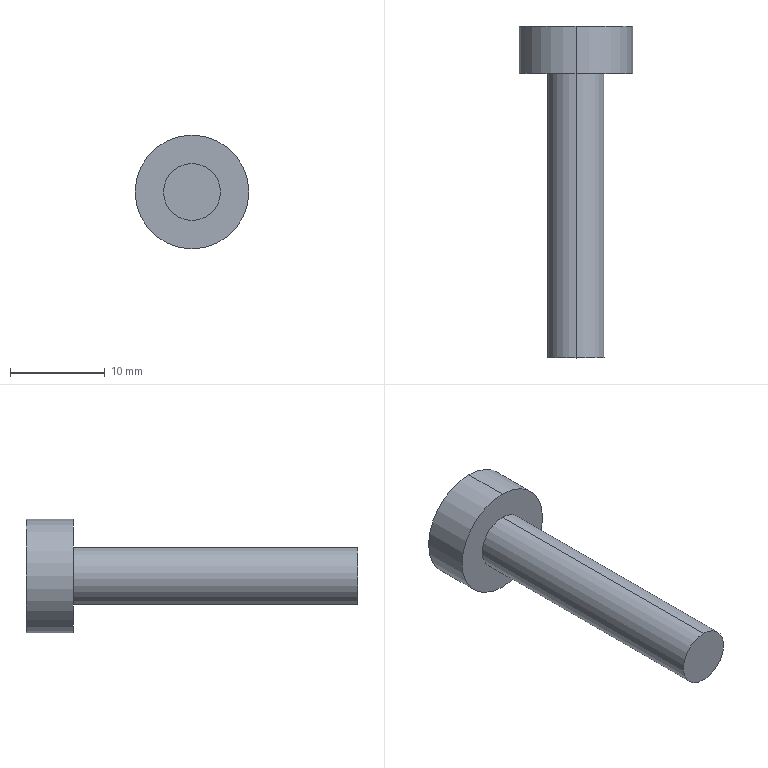Part | STEP file | 1 solid | 7 faces | box 12 x 35 x 12 mm | volume 1414 mm3 | cylinder 4 | plane 3 | commonest cylinder face diameters 6 x2 12 x2
STEP:
#1=CARTESIAN_POINT('',(0.,0.,0.));
#2=DIRECTION('',(0.,0.,1.));
#3=DIRECTION('',(1.,0.,0.));
#4=AXIS2_PLACEMENT_3D('',#1,#2,#3);
#5=CARTESIAN_POINT('',(0.,35.,-6.));
#6=VERTEX_POINT('',#5);
#7=CARTESIAN_POINT('',(0.,35.,6.));
#8=VERTEX_POINT('',#7);
#9=CARTESIAN_POINT('',(0.,35.,0.));
#10=DIRECTION('',(0.,-1.,0.));
#11=DIRECTION('',(0.,0.,-1.));
#12=AXIS2_PLACEMENT_3D('',#9,#10,#11);
#13=CIRCLE('',#12,6.);
#14=CARTESIAN_POINT('',(0.,0.,0.));
#15=DIRECTION('',(0.,-1.,0.));
#16=DIRECTION('',(0.,0.,-1.));
#17=AXIS2_PLACEMENT_3D('',#14,#15,#16);
#18=CYLINDRICAL_SURFACE('',#17,6.);
#19=CARTESIAN_POINT('',(0.,-35.));
#20=DIRECTION('',(1.,0.));
#21=VECTOR('',#20,1.);
#22=LINE('',#19,#21);
#23=(GEOMETRIC_REPRESENTATION_CONTEXT(2)PARAMETRIC_REPRESENTATION_CONTEXT()REPRESENTATION_CONTEXT('',''));
#24=DEFINITIONAL_REPRESENTATION('',(#22),#23);
#25=PCURVE('',#18,#24);
#26=CARTESIAN_POINT('',(6.,35.,0.));
#27=DIRECTION('',(0.,1.,0.));
#28=DIRECTION('',(0.,0.,1.));
#29=AXIS2_PLACEMENT_3D('',#26,#27,#28);
#30=PLANE('',#29);
#31=CARTESIAN_POINT('',(-6.,-6.));
#32=CARTESIAN_POINT('',(-6.,4.392));
#33=CARTESIAN_POINT('',(3.,-0.8038));
#34=CARTESIAN_POINT('',(12.,-6.));
#35=CARTESIAN_POINT('',(3.,-11.196));
#36=CARTESIAN_POINT('',(-6.,-16.392));
#37=CARTESIAN_POINT('',(-6.,-6.));
#38=(BOUNDED_CURVE()B_SPLINE_CURVE(2,(#31,#32,#33,#34,#35,#36,#37),.UNSPECIFIED.,.T.,.F.)B_SPLINE_CURVE_WITH_KNOTS((1,2,2,2,2,1),(-2.094,0.,2.094,4.189,6.283,8.378),.UNSPECIFIED.)CURVE()GEOMETRIC_REPRESENTATION_ITEM()RATIONAL_B_SPLINE_CURVE((1.,0.5,1.,0.5,1.,0.5,1.))REPRESENTATION_ITEM(''));
#39=(GEOMETRIC_REPRESENTATION_CONTEXT(2)PARAMETRIC_REPRESENTATION_CONTEXT()REPRESENTATION_CONTEXT('',''));
#40=DEFINITIONAL_REPRESENTATION('',(#38),#39);
#41=PCURVE('',#30,#40);
#42=SURFACE_CURVE('',#13,(#25,#41),.PCURVE_S1.);
#43=EDGE_CURVE('',#6,#8,#42,.T.);
#44=ORIENTED_EDGE('',*,*,#43,.T.);
#45=CARTESIAN_POINT('',(0.,30.,6.));
#46=VERTEX_POINT('',#45);
#47=CARTESIAN_POINT('',(0.,0.,6.));
#48=DIRECTION('',(0.,-1.,0.));
#49=VECTOR('',#48,1.);
#50=LINE('',#47,#49);
#51=CARTESIAN_POINT('',(3.142,0.));
#52=DIRECTION('',(0.,1.));
#53=VECTOR('',#52,1.);
#54=LINE('',#51,#53);
#55=(GEOMETRIC_REPRESENTATION_CONTEXT(2)PARAMETRIC_REPRESENTATION_CONTEXT()REPRESENTATION_CONTEXT('',''));
#56=DEFINITIONAL_REPRESENTATION('',(#54),#55);
#57=PCURVE('',#18,#56);
#58=CARTESIAN_POINT('',(0.,0.,0.));
#59=DIRECTION('',(0.,-1.,0.));
#60=DIRECTION('',(0.,0.,-1.));
#61=AXIS2_PLACEMENT_3D('',#58,#59,#60);
#62=CYLINDRICAL_SURFACE('',#61,6.);
#63=CARTESIAN_POINT('',(3.142,0.));
#64=DIRECTION('',(0.,1.));
#65=VECTOR('',#64,1.);
#66=LINE('',#63,#65);
#67=(GEOMETRIC_REPRESENTATION_CONTEXT(2)PARAMETRIC_REPRESENTATION_CONTEXT()REPRESENTATION_CONTEXT('',''));
#68=DEFINITIONAL_REPRESENTATION('',(#66),#67);
#69=PCURVE('',#62,#68);
#70=SURFACE_CURVE('',#50,(#57,#69),.PCURVE_S1.);
#71=EDGE_CURVE('',#8,#46,#70,.T.);
#72=ORIENTED_EDGE('',*,*,#71,.T.);
#73=CARTESIAN_POINT('',(0.,30.,-6.));
#74=VERTEX_POINT('',#73);
#75=CARTESIAN_POINT('',(0.,30.,0.));
#76=DIRECTION('',(0.,-1.,0.));
#77=DIRECTION('',(0.,0.,-1.));
#78=AXIS2_PLACEMENT_3D('',#75,#76,#77);
#79=CIRCLE('',#78,6.);
#80=CARTESIAN_POINT('',(0.,-30.));
#81=DIRECTION('',(1.,0.));
#82=VECTOR('',#81,1.);
#83=LINE('',#80,#82);
#84=(GEOMETRIC_REPRESENTATION_CONTEXT(2)PARAMETRIC_REPRESENTATION_CONTEXT()REPRESENTATION_CONTEXT('',''));
#85=DEFINITIONAL_REPRESENTATION('',(#83),#84);
#86=PCURVE('',#18,#85);
#87=CARTESIAN_POINT('',(3.,30.,0.));
#88=DIRECTION('',(0.,-1.,0.));
#89=DIRECTION('',(0.,0.,-1.));
#90=AXIS2_PLACEMENT_3D('',#87,#88,#89);
#91=PLANE('',#90);
#92=CARTESIAN_POINT('',(0.,-3.));
#93=DIRECTION('',(1.,0.));
#94=AXIS2_PLACEMENT_2D('',#92,#93);
#95=CIRCLE('',#94,6.);
#96=(GEOMETRIC_REPRESENTATION_CONTEXT(2)PARAMETRIC_REPRESENTATION_CONTEXT()REPRESENTATION_CONTEXT('',''));
#97=DEFINITIONAL_REPRESENTATION('',(#95),#96);
#98=PCURVE('',#91,#97);
#99=SURFACE_CURVE('',#79,(#86,#98),.PCURVE_S1.);
#100=EDGE_CURVE('',#74,#46,#99,.T.);
#101=ORIENTED_EDGE('',*,*,#100,.F.);
#102=CARTESIAN_POINT('',(0.,0.,-6.));
#103=DIRECTION('',(0.,-1.,0.));
#104=VECTOR('',#103,1.);
#105=LINE('',#102,#104);
#106=CARTESIAN_POINT('',(0.,0.));
#107=DIRECTION('',(0.,1.));
#108=VECTOR('',#107,1.);
#109=LINE('',#106,#108);
#110=(GEOMETRIC_REPRESENTATION_CONTEXT(2)PARAMETRIC_REPRESENTATION_CONTEXT()REPRESENTATION_CONTEXT('',''));
#111=DEFINITIONAL_REPRESENTATION('',(#109),#110);
#112=PCURVE('',#18,#111);
#113=CARTESIAN_POINT('',(6.283,0.));
#114=DIRECTION('',(0.,1.));
#115=VECTOR('',#114,1.);
#116=LINE('',#113,#115);
#117=(GEOMETRIC_REPRESENTATION_CONTEXT(2)PARAMETRIC_REPRESENTATION_CONTEXT()REPRESENTATION_CONTEXT('',''));
#118=DEFINITIONAL_REPRESENTATION('',(#116),#117);
#119=PCURVE('',#62,#118);
#120=SURFACE_CURVE('',#105,(#112,#119),.PCURVE_S1.);
#121=EDGE_CURVE('',#6,#74,#120,.T.);
#122=ORIENTED_EDGE('',*,*,#121,.F.);
#123=EDGE_LOOP('',(#44,#72,#101,#122));
#124=FACE_BOUND('',#123,.T.);
#125=ADVANCED_FACE('',(#124),#18,.T.);
#126=CARTESIAN_POINT('',(0.,30.,-3.));
#127=VERTEX_POINT('',#126);
#128=CARTESIAN_POINT('',(0.,30.,3.));
#129=VERTEX_POINT('',#128);
#130=CARTESIAN_POINT('',(0.,30.,0.));
#131=DIRECTION('',(0.,-1.,0.));
#132=DIRECTION('',(0.,0.,-1.));
#133=AXIS2_PLACEMENT_3D('',#130,#131,#132);
#134=CIRCLE('',#133,3.);
#135=CARTESIAN_POINT('',(0.,0.,0.));
#136=DIRECTION('',(0.,-1.,0.));
#137=DIRECTION('',(0.,0.,-1.));
#138=AXIS2_PLACEMENT_3D('',#135,#136,#137);
#139=CYLINDRICAL_SURFACE('',#138,3.);
#140=CARTESIAN_POINT('',(0.,-30.));
#141=DIRECTION('',(1.,0.));
#142=VECTOR('',#141,1.);
#143=LINE('',#140,#142);
#144=(GEOMETRIC_REPRESENTATION_CONTEXT(2)PARAMETRIC_REPRESENTATION_CONTEXT()REPRESENTATION_CONTEXT('',''));
#145=DEFINITIONAL_REPRESENTATION('',(#143),#144);
#146=PCURVE('',#139,#145);
#147=CARTESIAN_POINT('',(0.,-3.));
#148=DIRECTION('',(1.,0.));
#149=AXIS2_PLACEMENT_2D('',#147,#148);
#150=CIRCLE('',#149,3.);
#151=(GEOMETRIC_REPRESENTATION_CONTEXT(2)PARAMETRIC_REPRESENTATION_CONTEXT()REPRESENTATION_CONTEXT('',''));
#152=DEFINITIONAL_REPRESENTATION('',(#150),#151);
#153=PCURVE('',#91,#152);
#154=SURFACE_CURVE('',#134,(#146,#153),.PCURVE_S1.);
#155=EDGE_CURVE('',#127,#129,#154,.T.);
#156=ORIENTED_EDGE('',*,*,#155,.T.);
#157=CARTESIAN_POINT('',(0.,0.,3.));
#158=VERTEX_POINT('',#157);
#159=CARTESIAN_POINT('',(0.,0.,3.));
#160=DIRECTION('',(0.,-1.,0.));
#161=VECTOR('',#160,1.);
#162=LINE('',#159,#161);
#163=CARTESIAN_POINT('',(3.142,0.));
#164=DIRECTION('',(0.,1.));
#165=VECTOR('',#164,1.);
#166=LINE('',#163,#165);
#167=(GEOMETRIC_REPRESENTATION_CONTEXT(2)PARAMETRIC_REPRESENTATION_CONTEXT()REPRESENTATION_CONTEXT('',''));
#168=DEFINITIONAL_REPRESENTATION('',(#166),#167);
#169=PCURVE('',#139,#168);
#170=CARTESIAN_POINT('',(0.,0.,0.));
#171=DIRECTION('',(0.,-1.,0.));
#172=DIRECTION('',(0.,0.,-1.));
#173=AXIS2_PLACEMENT_3D('',#170,#171,#172);
#174=CYLINDRICAL_SURFACE('',#173,3.);
#175=CARTESIAN_POINT('',(3.142,0.));
#176=DIRECTION('',(0.,1.));
#177=VECTOR('',#176,1.);
#178=LINE('',#175,#177);
#179=(GEOMETRIC_REPRESENTATION_CONTEXT(2)PARAMETRIC_REPRESENTATION_CONTEXT()REPRESENTATION_CONTEXT('',''));
#180=DEFINITIONAL_REPRESENTATION('',(#178),#179);
#181=PCURVE('',#174,#180);
#182=SURFACE_CURVE('',#162,(#169,#181),.PCURVE_S1.);
#183=EDGE_CURVE('',#129,#158,#182,.T.);
#184=ORIENTED_EDGE('',*,*,#183,.T.);
#185=CARTESIAN_POINT('',(0.,0.,-3.));
#186=VERTEX_POINT('',#185);
#187=CARTESIAN_POINT('',(0.,0.,0.));
#188=DIRECTION('',(0.,-1.,0.));
#189=DIRECTION('',(0.,0.,-1.));
#190=AXIS2_PLACEMENT_3D('',#187,#188,#189);
#191=CIRCLE('',#190,3.);
#192=CARTESIAN_POINT('',(0.,0.));
#193=DIRECTION('',(1.,0.));
#194=VECTOR('',#193,1.);
#195=LINE('',#192,#194);
#196=(GEOMETRIC_REPRESENTATION_CONTEXT(2)PARAMETRIC_REPRESENTATION_CONTEXT()REPRESENTATION_CONTEXT('',''));
#197=DEFINITIONAL_REPRESENTATION('',(#195),#196);
#198=PCURVE('',#139,#197);
#199=CARTESIAN_POINT('',(0.,0.,0.));
#200=DIRECTION('',(0.,-1.,0.));
#201=DIRECTION('',(0.,0.,-1.));
#202=AXIS2_PLACEMENT_3D('',#199,#200,#201);
#203=PLANE('',#202);
#204=CARTESIAN_POINT('',(0.,0.));
#205=DIRECTION('',(1.,0.));
#206=AXIS2_PLACEMENT_2D('',#204,#205);
#207=CIRCLE('',#206,3.);
#208=(GEOMETRIC_REPRESENTATION_CONTEXT(2)PARAMETRIC_REPRESENTATION_CONTEXT()REPRESENTATION_CONTEXT('',''));
#209=DEFINITIONAL_REPRESENTATION('',(#207),#208);
#210=PCURVE('',#203,#209);
#211=SURFACE_CURVE('',#191,(#198,#210),.PCURVE_S1.);
#212=EDGE_CURVE('',#186,#158,#211,.T.);
#213=ORIENTED_EDGE('',*,*,#212,.F.);
#214=CARTESIAN_POINT('',(0.,0.,-3.));
#215=DIRECTION('',(0.,-1.,0.));
#216=VECTOR('',#215,1.);
#217=LINE('',#214,#216);
#218=CARTESIAN_POINT('',(0.,0.));
#219=DIRECTION('',(0.,1.));
#220=VECTOR('',#219,1.);
#221=LINE('',#218,#220);
#222=(GEOMETRIC_REPRESENTATION_CONTEXT(2)PARAMETRIC_REPRESENTATION_CONTEXT()REPRESENTATION_CONTEXT('',''));
#223=DEFINITIONAL_REPRESENTATION('',(#221),#222);
#224=PCURVE('',#139,#223);
#225=CARTESIAN_POINT('',(6.283,0.));
#226=DIRECTION('',(0.,1.));
#227=VECTOR('',#226,1.);
#228=LINE('',#225,#227);
#229=(GEOMETRIC_REPRESENTATION_CONTEXT(2)PARAMETRIC_REPRESENTATION_CONTEXT()REPRESENTATION_CONTEXT('',''));
#230=DEFINITIONAL_REPRESENTATION('',(#228),#229);
#231=PCURVE('',#174,#230);
#232=SURFACE_CURVE('',#217,(#224,#231),.PCURVE_S1.);
#233=EDGE_CURVE('',#127,#186,#232,.T.);
#234=ORIENTED_EDGE('',*,*,#233,.F.);
#235=EDGE_LOOP('',(#156,#184,#213,#234));
#236=FACE_BOUND('',#235,.T.);
#237=ADVANCED_FACE('',(#236),#139,.T.);
#238=ORIENTED_EDGE('',*,*,#212,.T.);
#239=CARTESIAN_POINT('',(0.,0.,0.));
#240=DIRECTION('',(0.,-1.,0.));
#241=DIRECTION('',(0.,0.,-1.));
#242=AXIS2_PLACEMENT_3D('',#239,#240,#241);
#243=CIRCLE('',#242,3.);
#244=CARTESIAN_POINT('',(0.,0.));
#245=DIRECTION('',(1.,0.));
#246=AXIS2_PLACEMENT_2D('',#244,#245);
#247=CIRCLE('',#246,3.);
#248=(GEOMETRIC_REPRESENTATION_CONTEXT(2)PARAMETRIC_REPRESENTATION_CONTEXT()REPRESENTATION_CONTEXT('',''));
#249=DEFINITIONAL_REPRESENTATION('',(#247),#248);
#250=PCURVE('',#203,#249);
#251=CARTESIAN_POINT('',(0.,0.));
#252=DIRECTION('',(1.,0.));
#253=VECTOR('',#252,1.);
#254=LINE('',#251,#253);
#255=(GEOMETRIC_REPRESENTATION_CONTEXT(2)PARAMETRIC_REPRESENTATION_CONTEXT()REPRESENTATION_CONTEXT('',''));
#256=DEFINITIONAL_REPRESENTATION('',(#254),#255);
#257=PCURVE('',#174,#256);
#258=SURFACE_CURVE('',#243,(#250,#257),.PCURVE_S1.);
#259=EDGE_CURVE('',#158,#186,#258,.T.);
#260=ORIENTED_EDGE('',*,*,#259,.T.);
#261=EDGE_LOOP('',(#238,#260));
#262=FACE_BOUND('',#261,.T.);
#263=ADVANCED_FACE('',(#262),#203,.T.);
#264=ORIENTED_EDGE('',*,*,#183,.F.);
#265=CARTESIAN_POINT('',(0.,30.,0.));
#266=DIRECTION('',(0.,-1.,0.));
#267=DIRECTION('',(0.,0.,-1.));
#268=AXIS2_PLACEMENT_3D('',#265,#266,#267);
#269=CIRCLE('',#268,3.);
#270=CARTESIAN_POINT('',(0.,-30.));
#271=DIRECTION('',(1.,0.));
#272=VECTOR('',#271,1.);
#273=LINE('',#270,#272);
#274=(GEOMETRIC_REPRESENTATION_CONTEXT(2)PARAMETRIC_REPRESENTATION_CONTEXT()REPRESENTATION_CONTEXT('',''));
#275=DEFINITIONAL_REPRESENTATION('',(#273),#274);
#276=PCURVE('',#174,#275);
#277=CARTESIAN_POINT('',(0.,-3.));
#278=DIRECTION('',(1.,0.));
#279=AXIS2_PLACEMENT_2D('',#277,#278);
#280=CIRCLE('',#279,3.);
#281=(GEOMETRIC_REPRESENTATION_CONTEXT(2)PARAMETRIC_REPRESENTATION_CONTEXT()REPRESENTATION_CONTEXT('',''));
#282=DEFINITIONAL_REPRESENTATION('',(#280),#281);
#283=PCURVE('',#91,#282);
#284=SURFACE_CURVE('',#269,(#276,#283),.PCURVE_S1.);
#285=EDGE_CURVE('',#129,#127,#284,.T.);
#286=ORIENTED_EDGE('',*,*,#285,.T.);
#287=ORIENTED_EDGE('',*,*,#233,.T.);
#288=ORIENTED_EDGE('',*,*,#259,.F.);
#289=EDGE_LOOP('',(#264,#286,#287,#288));
#290=FACE_BOUND('',#289,.T.);
#291=ADVANCED_FACE('',(#290),#174,.T.);
#292=ORIENTED_EDGE('',*,*,#100,.T.);
#293=CARTESIAN_POINT('',(0.,30.,0.));
#294=DIRECTION('',(0.,-1.,0.));
#295=DIRECTION('',(0.,0.,-1.));
#296=AXIS2_PLACEMENT_3D('',#293,#294,#295);
#297=CIRCLE('',#296,6.);
#298=CARTESIAN_POINT('',(0.,-3.));
#299=DIRECTION('',(1.,0.));
#300=AXIS2_PLACEMENT_2D('',#298,#299);
#301=CIRCLE('',#300,6.);
#302=(GEOMETRIC_REPRESENTATION_CONTEXT(2)PARAMETRIC_REPRESENTATION_CONTEXT()REPRESENTATION_CONTEXT('',''));
#303=DEFINITIONAL_REPRESENTATION('',(#301),#302);
#304=PCURVE('',#91,#303);
#305=CARTESIAN_POINT('',(0.,-30.));
#306=DIRECTION('',(1.,0.));
#307=VECTOR('',#306,1.);
#308=LINE('',#305,#307);
#309=(GEOMETRIC_REPRESENTATION_CONTEXT(2)PARAMETRIC_REPRESENTATION_CONTEXT()REPRESENTATION_CONTEXT('',''));
#310=DEFINITIONAL_REPRESENTATION('',(#308),#309);
#311=PCURVE('',#62,#310);
#312=SURFACE_CURVE('',#297,(#304,#311),.PCURVE_S1.);
#313=EDGE_CURVE('',#46,#74,#312,.T.);
#314=ORIENTED_EDGE('',*,*,#313,.T.);
#315=EDGE_LOOP('',(#292,#314));
#316=FACE_BOUND('',#315,.T.);
#317=ORIENTED_EDGE('',*,*,#155,.F.);
#318=ORIENTED_EDGE('',*,*,#285,.F.);
#319=EDGE_LOOP('',(#317,#318));
#320=FACE_BOUND('',#319,.T.);
#321=ADVANCED_FACE('',(#316,#320),#91,.T.);
#322=ORIENTED_EDGE('',*,*,#71,.F.);
#323=CARTESIAN_POINT('',(0.,35.,0.));
#324=DIRECTION('',(0.,-1.,0.));
#325=DIRECTION('',(0.,0.,-1.));
#326=AXIS2_PLACEMENT_3D('',#323,#324,#325);
#327=CIRCLE('',#326,6.);
#328=CARTESIAN_POINT('',(0.,-35.));
#329=DIRECTION('',(1.,0.));
#330=VECTOR('',#329,1.);
#331=LINE('',#328,#330);
#332=(GEOMETRIC_REPRESENTATION_CONTEXT(2)PARAMETRIC_REPRESENTATION_CONTEXT()REPRESENTATION_CONTEXT('',''));
#333=DEFINITIONAL_REPRESENTATION('',(#331),#332);
#334=PCURVE('',#62,#333);
#335=CARTESIAN_POINT('',(-6.,-6.));
#336=CARTESIAN_POINT('',(-6.,4.392));
#337=CARTESIAN_POINT('',(3.,-0.8038));
#338=CARTESIAN_POINT('',(12.,-6.));
#339=CARTESIAN_POINT('',(3.,-11.196));
#340=CARTESIAN_POINT('',(-6.,-16.392));
#341=CARTESIAN_POINT('',(-6.,-6.));
#342=(BOUNDED_CURVE()B_SPLINE_CURVE(2,(#335,#336,#337,#338,#339,#340,#341),.UNSPECIFIED.,.T.,.F.)B_SPLINE_CURVE_WITH_KNOTS((1,2,2,2,2,1),(-2.094,0.,2.094,4.189,6.283,8.378),.UNSPECIFIED.)CURVE()GEOMETRIC_REPRESENTATION_ITEM()RATIONAL_B_SPLINE_CURVE((1.,0.5,1.,0.5,1.,0.5,1.))REPRESENTATION_ITEM(''));
#343=(GEOMETRIC_REPRESENTATION_CONTEXT(2)PARAMETRIC_REPRESENTATION_CONTEXT()REPRESENTATION_CONTEXT('',''));
#344=DEFINITIONAL_REPRESENTATION('',(#342),#343);
#345=PCURVE('',#30,#344);
#346=SURFACE_CURVE('',#327,(#334,#345),.PCURVE_S1.);
#347=EDGE_CURVE('',#8,#6,#346,.T.);
#348=ORIENTED_EDGE('',*,*,#347,.T.);
#349=ORIENTED_EDGE('',*,*,#121,.T.);
#350=ORIENTED_EDGE('',*,*,#313,.F.);
#351=EDGE_LOOP('',(#322,#348,#349,#350));
#352=FACE_BOUND('',#351,.T.);
#353=ADVANCED_FACE('',(#352),#62,.T.);
#354=ORIENTED_EDGE('',*,*,#43,.F.);
#355=ORIENTED_EDGE('',*,*,#347,.F.);
#356=EDGE_LOOP('',(#354,#355));
#357=FACE_BOUND('',#356,.T.);
#358=ADVANCED_FACE('',(#357),#30,.T.);
#359=CLOSED_SHELL('',(#125,#237,#263,#291,#321,#353,#358));
#360=MANIFOLD_SOLID_BREP('',#359);
#361=(LENGTH_UNIT()NAMED_UNIT(*)SI_UNIT(.MILLI.,.METRE.));
#362=UNCERTAINTY_MEASURE_WITH_UNIT(LENGTH_MEASURE(0.0000001),#361,'','');
#363=(NAMED_UNIT(*)PLANE_ANGLE_UNIT()SI_UNIT($,.RADIAN.));
#364=(NAMED_UNIT(*)SI_UNIT($,.STERADIAN.)SOLID_ANGLE_UNIT());
#365=(GEOMETRIC_REPRESENTATION_CONTEXT(3)GLOBAL_UNCERTAINTY_ASSIGNED_CONTEXT((#362))GLOBAL_UNIT_ASSIGNED_CONTEXT((#361,#363,#364))REPRESENTATION_CONTEXT('',''));
#366=ADVANCED_BREP_SHAPE_REPRESENTATION('',(#4,#360),#365);